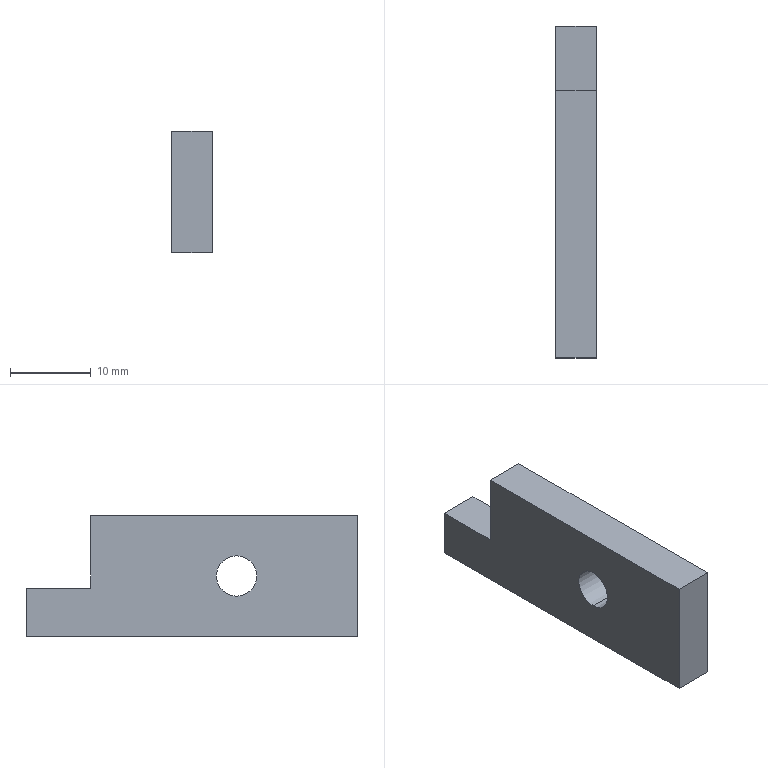Part | SolidWorks | features ICE 2, MBimport 1 | 1 solid | 10 faces | box 5 x 41 x 15 mm | volume 2617 mm3 | plane 8 | cylinder 2 | commonest cylinder face diameters 5 x2
STEP:
#1=CARTESIAN_POINT('',(0.,26.,-7.5));
#2=VERTEX_POINT('',#1);
#3=CARTESIAN_POINT('',(0.,26.,-1.5));
#4=VERTEX_POINT('',#3);
#5=CARTESIAN_POINT('',(0.,26.,-7.5));
#6=DIRECTION('',(0.,0.,1.));
#7=VECTOR('',#6,1000.);
#8=LINE('',#5,#7);
#9=EDGE_CURVE('',#2,#4,#8,.T.);
#10=ORIENTED_EDGE('',*,*,#9,.T.);
#11=CARTESIAN_POINT('',(5.,26.,-1.5));
#12=VERTEX_POINT('',#11);
#13=CARTESIAN_POINT('',(0.,26.,-1.5));
#14=DIRECTION('',(-1.,0.,0.));
#15=VECTOR('',#14,1000.);
#16=LINE('',#13,#15);
#17=EDGE_CURVE('',#12,#4,#16,.T.);
#18=ORIENTED_EDGE('',*,*,#17,.F.);
#19=CARTESIAN_POINT('',(5.,26.,-7.5));
#20=VERTEX_POINT('',#19);
#21=CARTESIAN_POINT('',(5.,26.,7.5));
#22=DIRECTION('',(0.,0.,-1.));
#23=VECTOR('',#22,1000.);
#24=LINE('',#21,#23);
#25=EDGE_CURVE('',#12,#20,#24,.T.);
#26=ORIENTED_EDGE('',*,*,#25,.T.);
#27=CARTESIAN_POINT('',(5.,26.,-7.5));
#28=DIRECTION('',(-1.,0.,0.));
#29=VECTOR('',#28,1000.);
#30=LINE('',#27,#29);
#31=EDGE_CURVE('',#20,#2,#30,.T.);
#32=ORIENTED_EDGE('',*,*,#31,.T.);
#33=EDGE_LOOP('',(#10,#18,#26,#32));
#34=FACE_OUTER_BOUND('',#33,.T.);
#35=CARTESIAN_POINT('',(0.,26.,0.));
#36=DIRECTION('',(0.,1.,0.));
#37=DIRECTION('',(0.,0.,1.));
#38=AXIS2_PLACEMENT_3D('',#35,#36,#37);
#39=PLANE('',#38);
#40=ADVANCED_FACE('',(#34),#39,.T.);
#41=CARTESIAN_POINT('',(0.,-15.,7.5));
#42=VERTEX_POINT('',#41);
#43=CARTESIAN_POINT('',(0.,18.,7.5));
#44=VERTEX_POINT('',#43);
#45=CARTESIAN_POINT('',(0.,-15.,7.5));
#46=DIRECTION('',(0.,1.,0.));
#47=VECTOR('',#46,1000.);
#48=LINE('',#45,#47);
#49=EDGE_CURVE('',#42,#44,#48,.T.);
#50=ORIENTED_EDGE('',*,*,#49,.T.);
#51=CARTESIAN_POINT('',(0.,18.,-1.5));
#52=VERTEX_POINT('',#51);
#53=CARTESIAN_POINT('',(0.,18.,-1.5));
#54=DIRECTION('',(0.,0.,1.));
#55=VECTOR('',#54,1000.);
#56=LINE('',#53,#55);
#57=EDGE_CURVE('',#52,#44,#56,.T.);
#58=ORIENTED_EDGE('',*,*,#57,.F.);
#59=CARTESIAN_POINT('',(0.,26.,-1.5));
#60=DIRECTION('',(0.,-1.,0.));
#61=VECTOR('',#60,1000.);
#62=LINE('',#59,#61);
#63=EDGE_CURVE('',#4,#52,#62,.T.);
#64=ORIENTED_EDGE('',*,*,#63,.F.);
#65=ORIENTED_EDGE('',*,*,#9,.F.);
#66=CARTESIAN_POINT('',(0.,-15.,-7.5));
#67=VERTEX_POINT('',#66);
#68=CARTESIAN_POINT('',(0.,20.,-7.5));
#69=DIRECTION('',(0.,-1.,0.));
#70=VECTOR('',#69,1000.);
#71=LINE('',#68,#70);
#72=EDGE_CURVE('',#2,#67,#71,.T.);
#73=ORIENTED_EDGE('',*,*,#72,.T.);
#74=CARTESIAN_POINT('',(0.,-15.,7.5));
#75=DIRECTION('',(0.,0.,-1.));
#76=VECTOR('',#75,1000.);
#77=LINE('',#74,#76);
#78=EDGE_CURVE('',#42,#67,#77,.T.);
#79=ORIENTED_EDGE('',*,*,#78,.F.);
#80=EDGE_LOOP('',(#50,#58,#64,#65,#73,#79));
#81=FACE_OUTER_BOUND('',#80,.T.);
#82=CARTESIAN_POINT('',(0.,0.,2.5));
#83=VERTEX_POINT('',#82);
#84=CARTESIAN_POINT('',(0.,0.,-2.5));
#85=VERTEX_POINT('',#84);
#86=CARTESIAN_POINT('',(0.,0.,0.));
#87=DIRECTION('',(1.,0.,0.));
#88=DIRECTION('',(0.,0.,1.));
#89=AXIS2_PLACEMENT_3D('',#86,#87,#88);
#90=CIRCLE('',#89,2.5);
#91=EDGE_CURVE('',#83,#85,#90,.T.);
#92=ORIENTED_EDGE('',*,*,#91,.T.);
#93=CARTESIAN_POINT('',(0.,0.,0.));
#94=DIRECTION('',(1.,0.,0.));
#95=DIRECTION('',(0.,0.,-1.));
#96=AXIS2_PLACEMENT_3D('',#93,#94,#95);
#97=CIRCLE('',#96,2.5);
#98=EDGE_CURVE('',#85,#83,#97,.T.);
#99=ORIENTED_EDGE('',*,*,#98,.T.);
#100=EDGE_LOOP('',(#92,#99));
#101=FACE_BOUND('',#100,.T.);
#102=CARTESIAN_POINT('',(0.,0.,0.));
#103=DIRECTION('',(1.,0.,0.));
#104=DIRECTION('',(0.,1.,0.));
#105=AXIS2_PLACEMENT_3D('',#102,#103,#104);
#106=PLANE('',#105);
#107=ADVANCED_FACE('',(#81,#101),#106,.F.);
#108=CARTESIAN_POINT('',(5.,-15.,-7.5));
#109=VERTEX_POINT('',#108);
#110=CARTESIAN_POINT('',(0.,-15.,-7.5));
#111=DIRECTION('',(1.,0.,0.));
#112=VECTOR('',#111,1000.);
#113=LINE('',#110,#112);
#114=EDGE_CURVE('',#67,#109,#113,.T.);
#115=ORIENTED_EDGE('',*,*,#114,.T.);
#116=CARTESIAN_POINT('',(5.,-15.,7.5));
#117=VERTEX_POINT('',#116);
#118=CARTESIAN_POINT('',(5.,-15.,7.5));
#119=DIRECTION('',(0.,0.,-1.));
#120=VECTOR('',#119,1000.);
#121=LINE('',#118,#120);
#122=EDGE_CURVE('',#117,#109,#121,.T.);
#123=ORIENTED_EDGE('',*,*,#122,.F.);
#124=CARTESIAN_POINT('',(0.,-15.,7.5));
#125=DIRECTION('',(1.,0.,0.));
#126=VECTOR('',#125,1000.);
#127=LINE('',#124,#126);
#128=EDGE_CURVE('',#42,#117,#127,.T.);
#129=ORIENTED_EDGE('',*,*,#128,.F.);
#130=ORIENTED_EDGE('',*,*,#78,.T.);
#131=EDGE_LOOP('',(#115,#123,#129,#130));
#132=FACE_OUTER_BOUND('',#131,.T.);
#133=CARTESIAN_POINT('',(0.,-15.,7.5));
#134=DIRECTION('',(0.,-1.,0.));
#135=DIRECTION('',(0.,0.,-1.));
#136=AXIS2_PLACEMENT_3D('',#133,#134,#135);
#137=PLANE('',#136);
#138=ADVANCED_FACE('',(#132),#137,.T.);
#139=CARTESIAN_POINT('',(5.,18.,7.5));
#140=VERTEX_POINT('',#139);
#141=CARTESIAN_POINT('',(0.,18.,7.5));
#142=DIRECTION('',(1.,0.,0.));
#143=VECTOR('',#142,1000.);
#144=LINE('',#141,#143);
#145=EDGE_CURVE('',#44,#140,#144,.T.);
#146=ORIENTED_EDGE('',*,*,#145,.F.);
#147=ORIENTED_EDGE('',*,*,#49,.F.);
#148=ORIENTED_EDGE('',*,*,#128,.T.);
#149=CARTESIAN_POINT('',(5.,-15.,7.5));
#150=DIRECTION('',(0.,1.,0.));
#151=VECTOR('',#150,1000.);
#152=LINE('',#149,#151);
#153=EDGE_CURVE('',#117,#140,#152,.T.);
#154=ORIENTED_EDGE('',*,*,#153,.T.);
#155=EDGE_LOOP('',(#146,#147,#148,#154));
#156=FACE_OUTER_BOUND('',#155,.T.);
#157=CARTESIAN_POINT('',(0.,15.,7.5));
#158=DIRECTION('',(0.,0.,1.));
#159=DIRECTION('',(0.,-1.,0.));
#160=AXIS2_PLACEMENT_3D('',#157,#158,#159);
#161=PLANE('',#160);
#162=ADVANCED_FACE('',(#156),#161,.T.);
#163=ORIENTED_EDGE('',*,*,#114,.F.);
#164=ORIENTED_EDGE('',*,*,#72,.F.);
#165=ORIENTED_EDGE('',*,*,#31,.F.);
#166=CARTESIAN_POINT('',(5.,-15.,-7.5));
#167=DIRECTION('',(0.,1.,0.));
#168=VECTOR('',#167,1000.);
#169=LINE('',#166,#168);
#170=EDGE_CURVE('',#109,#20,#169,.T.);
#171=ORIENTED_EDGE('',*,*,#170,.F.);
#172=EDGE_LOOP('',(#163,#164,#165,#171));
#173=FACE_OUTER_BOUND('',#172,.T.);
#174=CARTESIAN_POINT('',(0.,-15.,-7.5));
#175=DIRECTION('',(0.,0.,-1.));
#176=DIRECTION('',(0.,1.,0.));
#177=AXIS2_PLACEMENT_3D('',#174,#175,#176);
#178=PLANE('',#177);
#179=ADVANCED_FACE('',(#173),#178,.T.);
#180=CARTESIAN_POINT('',(5.,0.,2.5));
#181=VERTEX_POINT('',#180);
#182=CARTESIAN_POINT('',(5.,0.,2.5));
#183=DIRECTION('',(-1.,0.,0.));
#184=VECTOR('',#183,1000.);
#185=LINE('',#182,#184);
#186=EDGE_CURVE('',#181,#83,#185,.T.);
#187=ORIENTED_EDGE('',*,*,#186,.F.);
#188=CARTESIAN_POINT('',(5.,0.,-2.5));
#189=VERTEX_POINT('',#188);
#190=CARTESIAN_POINT('',(5.,0.,0.));
#191=DIRECTION('',(1.,0.,0.));
#192=DIRECTION('',(0.,0.,1.));
#193=AXIS2_PLACEMENT_3D('',#190,#191,#192);
#194=CIRCLE('',#193,2.5);
#195=EDGE_CURVE('',#181,#189,#194,.T.);
#196=ORIENTED_EDGE('',*,*,#195,.T.);
#197=CARTESIAN_POINT('',(5.,0.,-2.5));
#198=DIRECTION('',(-1.,0.,0.));
#199=VECTOR('',#198,1000.);
#200=LINE('',#197,#199);
#201=EDGE_CURVE('',#189,#85,#200,.T.);
#202=ORIENTED_EDGE('',*,*,#201,.T.);
#203=ORIENTED_EDGE('',*,*,#91,.F.);
#204=EDGE_LOOP('',(#187,#196,#202,#203));
#205=FACE_OUTER_BOUND('',#204,.T.);
#206=CARTESIAN_POINT('',(5.,0.,0.));
#207=DIRECTION('',(-1.,0.,0.));
#208=DIRECTION('',(0.,0.,-1.));
#209=AXIS2_PLACEMENT_3D('',#206,#207,#208);
#210=CYLINDRICAL_SURFACE('',#209,2.5);
#211=ADVANCED_FACE('',(#205),#210,.F.);
#212=ORIENTED_EDGE('',*,*,#201,.F.);
#213=CARTESIAN_POINT('',(5.,0.,0.));
#214=DIRECTION('',(1.,0.,0.));
#215=DIRECTION('',(0.,0.,-1.));
#216=AXIS2_PLACEMENT_3D('',#213,#214,#215);
#217=CIRCLE('',#216,2.5);
#218=EDGE_CURVE('',#189,#181,#217,.T.);
#219=ORIENTED_EDGE('',*,*,#218,.T.);
#220=ORIENTED_EDGE('',*,*,#186,.T.);
#221=ORIENTED_EDGE('',*,*,#98,.F.);
#222=EDGE_LOOP('',(#212,#219,#220,#221));
#223=FACE_OUTER_BOUND('',#222,.T.);
#224=CARTESIAN_POINT('',(5.,0.,0.));
#225=DIRECTION('',(-1.,0.,0.));
#226=DIRECTION('',(0.,0.,-1.));
#227=AXIS2_PLACEMENT_3D('',#224,#225,#226);
#228=CYLINDRICAL_SURFACE('',#227,2.5);
#229=ADVANCED_FACE('',(#223),#228,.F.);
#230=CARTESIAN_POINT('',(5.,18.,-1.5));
#231=VERTEX_POINT('',#230);
#232=CARTESIAN_POINT('',(5.,18.,-1.5));
#233=DIRECTION('',(0.,0.,1.));
#234=VECTOR('',#233,1000.);
#235=LINE('',#232,#234);
#236=EDGE_CURVE('',#231,#140,#235,.T.);
#237=ORIENTED_EDGE('',*,*,#236,.T.);
#238=ORIENTED_EDGE('',*,*,#153,.F.);
#239=ORIENTED_EDGE('',*,*,#122,.T.);
#240=ORIENTED_EDGE('',*,*,#170,.T.);
#241=ORIENTED_EDGE('',*,*,#25,.F.);
#242=CARTESIAN_POINT('',(5.,26.,-1.5));
#243=DIRECTION('',(0.,1.,0.));
#244=VECTOR('',#243,1000.);
#245=LINE('',#242,#244);
#246=EDGE_CURVE('',#231,#12,#245,.T.);
#247=ORIENTED_EDGE('',*,*,#246,.F.);
#248=EDGE_LOOP('',(#237,#238,#239,#240,#241,#247));
#249=FACE_OUTER_BOUND('',#248,.T.);
#250=ORIENTED_EDGE('',*,*,#195,.F.);
#251=ORIENTED_EDGE('',*,*,#218,.F.);
#252=EDGE_LOOP('',(#250,#251));
#253=FACE_BOUND('',#252,.T.);
#254=CARTESIAN_POINT('',(5.,0.,0.));
#255=DIRECTION('',(1.,0.,0.));
#256=DIRECTION('',(0.,1.,0.));
#257=AXIS2_PLACEMENT_3D('',#254,#255,#256);
#258=PLANE('',#257);
#259=ADVANCED_FACE('',(#249,#253),#258,.T.);
#260=ORIENTED_EDGE('',*,*,#145,.T.);
#261=ORIENTED_EDGE('',*,*,#236,.F.);
#262=CARTESIAN_POINT('',(0.,18.,-1.5));
#263=DIRECTION('',(1.,0.,0.));
#264=VECTOR('',#263,1000.);
#265=LINE('',#262,#264);
#266=EDGE_CURVE('',#52,#231,#265,.T.);
#267=ORIENTED_EDGE('',*,*,#266,.F.);
#268=ORIENTED_EDGE('',*,*,#57,.T.);
#269=EDGE_LOOP('',(#260,#261,#267,#268));
#270=FACE_OUTER_BOUND('',#269,.T.);
#271=CARTESIAN_POINT('',(0.,18.,-1.5));
#272=DIRECTION('',(0.,-1.,0.));
#273=DIRECTION('',(0.,0.,-1.));
#274=AXIS2_PLACEMENT_3D('',#271,#272,#273);
#275=PLANE('',#274);
#276=ADVANCED_FACE('',(#270),#275,.F.);
#277=ORIENTED_EDGE('',*,*,#63,.T.);
#278=ORIENTED_EDGE('',*,*,#266,.T.);
#279=ORIENTED_EDGE('',*,*,#246,.T.);
#280=ORIENTED_EDGE('',*,*,#17,.T.);
#281=EDGE_LOOP('',(#277,#278,#279,#280));
#282=FACE_OUTER_BOUND('',#281,.T.);
#283=CARTESIAN_POINT('',(0.,0.,-1.5));
#284=DIRECTION('',(0.,0.,1.));
#285=DIRECTION('',(1.,0.,0.));
#286=AXIS2_PLACEMENT_3D('',#283,#284,#285);
#287=PLANE('',#286);
#288=ADVANCED_FACE('',(#282),#287,.T.);
#289=CLOSED_SHELL('',(#40,#107,#138,#162,#179,#211,#229,#259,#276,#288));
#290=MANIFOLD_SOLID_BREP('',#289);
#291=CARTESIAN_POINT('',(0.,0.,0.));
#292=DIRECTION('',(0.,0.,1.));
#293=DIRECTION('',(1.,0.,0.));
#294=AXIS2_PLACEMENT_3D('',#291,#292,#293);
#295=(LENGTH_UNIT()NAMED_UNIT(*)SI_UNIT(.MILLI.,.METRE.));
#296=UNCERTAINTY_MEASURE_WITH_UNIT(LENGTH_MEASURE(0.00001),#295,'','');
#297=(NAMED_UNIT(*)PLANE_ANGLE_UNIT()SI_UNIT($,.RADIAN.));
#298=(NAMED_UNIT(*)SI_UNIT($,.STERADIAN.)SOLID_ANGLE_UNIT());
#299=(GEOMETRIC_REPRESENTATION_CONTEXT(3)GLOBAL_UNCERTAINTY_ASSIGNED_CONTEXT((#296))GLOBAL_UNIT_ASSIGNED_CONTEXT((#295,#297,#298))REPRESENTATION_CONTEXT('',''));
#300=ADVANCED_BREP_SHAPE_REPRESENTATION('',(#290,#294),#299);